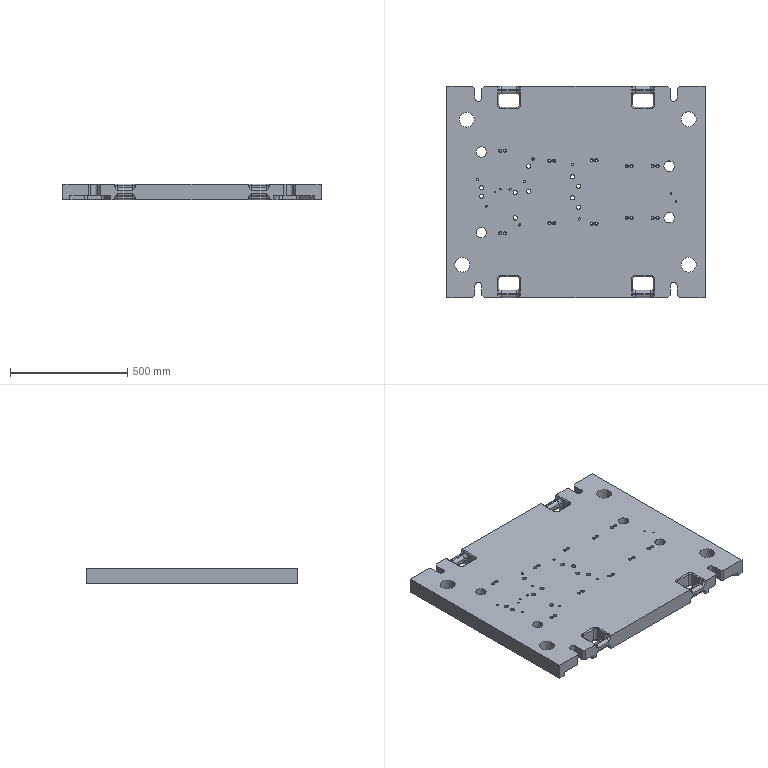Part | STEP file | 1_id194_x_t | 1 solid | 643 faces | box 1100 x 900 x 68 mm | volume 61756631 mm3 | cylinder 297 | plane 144 | cone 122 | torus 48 | spline 32 | commonest cylinder face diameters 10 x56 25.4 x48 6.528 x28 7.938 x25 9 x20 14 x20